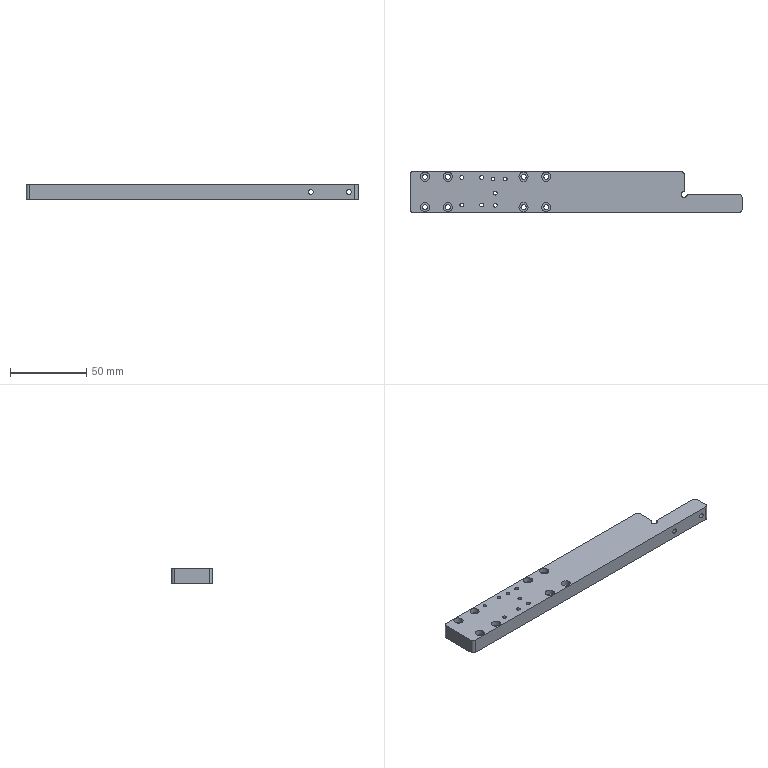Part | STEP file | FBDS-CS-023 | 1 solid | 86 faces | box 218 x 27 x 10 mm | volume 50909 mm3 | cylinder 64 | plane 16 | cone 6 | commonest cylinder face diameters 2.5 x16 3.4 x16 6 x16 3.3 x10 4 x6